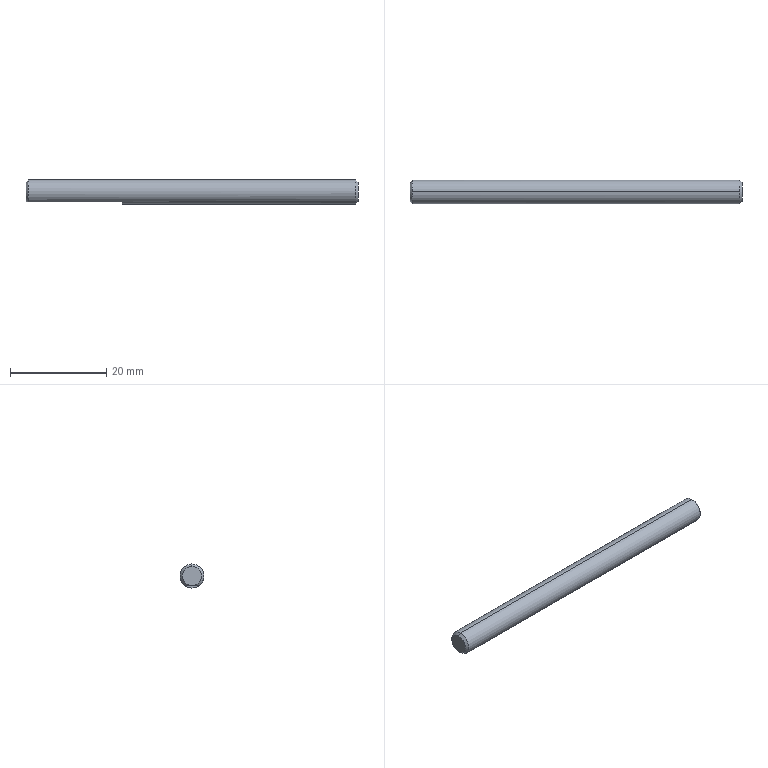Part | SolidWorks | features BaseBody 1 | 1 solid | 10 faces | box 69 x 5 x 5 mm | volume 1331 mm3 | cone 4 | plane 4 | cylinder 2 | commonest cylinder face diameters 5 x2
STEP:
#1=CARTESIAN_POINT('',(69.,0.,-2.));
#2=VERTEX_POINT('',#1);
#3=CARTESIAN_POINT('',(69.,0.,2.));
#4=VERTEX_POINT('',#3);
#5=CARTESIAN_POINT('',(69.,0.,0.));
#6=DIRECTION('',(1.,0.,0.));
#7=DIRECTION('',(0.,0.,1.));
#8=AXIS2_PLACEMENT_3D('',#5,#6,#7);
#9=CIRCLE('',#8,2.);
#10=EDGE_CURVE('',#2,#4,#9,.T.);
#11=ORIENTED_EDGE('',*,*,#10,.F.);
#12=CARTESIAN_POINT('',(68.5,0.,-2.5));
#13=VERTEX_POINT('',#12);
#14=CARTESIAN_POINT('',(69.,0.,-2.));
#15=DIRECTION('',(-0.7071,0.,-0.7071));
#16=VECTOR('',#15,1000.);
#17=LINE('',#14,#16);
#18=EDGE_CURVE('',#2,#13,#17,.T.);
#19=ORIENTED_EDGE('',*,*,#18,.T.);
#20=CARTESIAN_POINT('',(68.5,0.,2.5));
#21=VERTEX_POINT('',#20);
#22=CARTESIAN_POINT('',(68.5,0.,0.));
#23=DIRECTION('',(-1.,0.,0.));
#24=DIRECTION('',(0.,0.,1.));
#25=AXIS2_PLACEMENT_3D('',#22,#23,#24);
#26=CIRCLE('',#25,2.5);
#27=EDGE_CURVE('',#21,#13,#26,.T.);
#28=ORIENTED_EDGE('',*,*,#27,.F.);
#29=CARTESIAN_POINT('',(69.,0.,2.));
#30=DIRECTION('',(-0.7071,0.,0.7071));
#31=VECTOR('',#30,1000.);
#32=LINE('',#29,#31);
#33=EDGE_CURVE('',#4,#21,#32,.T.);
#34=ORIENTED_EDGE('',*,*,#33,.F.);
#35=EDGE_LOOP('',(#11,#19,#28,#34));
#36=FACE_OUTER_BOUND('',#35,.T.);
#37=CARTESIAN_POINT('',(69.,0.,0.));
#38=DIRECTION('',(-1.,0.,0.));
#39=DIRECTION('',(0.,0.,1.));
#40=AXIS2_PLACEMENT_3D('',#37,#38,#39);
#41=CONICAL_SURFACE('',#40,2.,0.7854);
#42=ADVANCED_FACE('',(#36),#41,.T.);
#43=ORIENTED_EDGE('',*,*,#27,.T.);
#44=CARTESIAN_POINT('',(20.,0.,-2.5));
#45=VERTEX_POINT('',#44);
#46=CARTESIAN_POINT('',(68.5,0.,-2.5));
#47=DIRECTION('',(-1.,0.,0.));
#48=VECTOR('',#47,1000.);
#49=LINE('',#46,#48);
#50=EDGE_CURVE('',#13,#45,#49,.T.);
#51=ORIENTED_EDGE('',*,*,#50,.T.);
#52=CARTESIAN_POINT('',(20.,1.5,-2.));
#53=VERTEX_POINT('',#52);
#54=CARTESIAN_POINT('',(20.,0.,0.));
#55=DIRECTION('',(-1.,0.,0.));
#56=DIRECTION('',(0.,0.,1.));
#57=AXIS2_PLACEMENT_3D('',#54,#55,#56);
#58=CIRCLE('',#57,2.5);
#59=EDGE_CURVE('',#53,#45,#58,.T.);
#60=ORIENTED_EDGE('',*,*,#59,.F.);
#61=CARTESIAN_POINT('',(0.5,1.5,-2.));
#62=VERTEX_POINT('',#61);
#63=CARTESIAN_POINT('',(34.5,1.5,-2.));
#64=DIRECTION('',(1.,0.,0.));
#65=VECTOR('',#64,1000.);
#66=LINE('',#63,#65);
#67=EDGE_CURVE('',#62,#53,#66,.T.);
#68=ORIENTED_EDGE('',*,*,#67,.F.);
#69=CARTESIAN_POINT('',(0.5,0.,2.5));
#70=VERTEX_POINT('',#69);
#71=CARTESIAN_POINT('',(0.5,0.,0.));
#72=DIRECTION('',(-1.,0.,0.));
#73=DIRECTION('',(0.,0.,1.));
#74=AXIS2_PLACEMENT_3D('',#71,#72,#73);
#75=CIRCLE('',#74,2.5);
#76=EDGE_CURVE('',#70,#62,#75,.T.);
#77=ORIENTED_EDGE('',*,*,#76,.F.);
#78=CARTESIAN_POINT('',(68.5,0.,2.5));
#79=DIRECTION('',(-1.,0.,0.));
#80=VECTOR('',#79,1000.);
#81=LINE('',#78,#80);
#82=EDGE_CURVE('',#21,#70,#81,.T.);
#83=ORIENTED_EDGE('',*,*,#82,.F.);
#84=EDGE_LOOP('',(#43,#51,#60,#68,#77,#83));
#85=FACE_OUTER_BOUND('',#84,.T.);
#86=CARTESIAN_POINT('',(68.5,0.,0.));
#87=DIRECTION('',(-1.,0.,0.));
#88=DIRECTION('',(0.,0.,1.));
#89=AXIS2_PLACEMENT_3D('',#86,#87,#88);
#90=CYLINDRICAL_SURFACE('',#89,2.5);
#91=ADVANCED_FACE('',(#85),#90,.T.);
#92=CARTESIAN_POINT('',(0.,0.,2.));
#93=VERTEX_POINT('',#92);
#94=CARTESIAN_POINT('',(0.,0.,-2.));
#95=VERTEX_POINT('',#94);
#96=CARTESIAN_POINT('',(0.,0.,0.));
#97=DIRECTION('',(-1.,0.,0.));
#98=DIRECTION('',(0.,0.,-1.));
#99=AXIS2_PLACEMENT_3D('',#96,#97,#98);
#100=CIRCLE('',#99,2.);
#101=EDGE_CURVE('',#93,#95,#100,.T.);
#102=ORIENTED_EDGE('',*,*,#101,.F.);
#103=CARTESIAN_POINT('',(0.,0.,2.));
#104=DIRECTION('',(0.7071,0.,0.7071));
#105=VECTOR('',#104,1000.);
#106=LINE('',#103,#105);
#107=EDGE_CURVE('',#93,#70,#106,.T.);
#108=ORIENTED_EDGE('',*,*,#107,.T.);
#109=ORIENTED_EDGE('',*,*,#76,.T.);
#110=CARTESIAN_POINT('',(0.5,1.5,-2.));
#111=CARTESIAN_POINT('',(0.4247,1.374,-2.));
#112=CARTESIAN_POINT('',(0.3577,1.253,-2.));
#113=CARTESIAN_POINT('',(0.2697,1.074,-2.));
#114=CARTESIAN_POINT('',(0.2425,1.016,-2.));
#115=CARTESIAN_POINT('',(0.2048,0.9284,-2.));
#116=CARTESIAN_POINT('',(0.1867,0.8849,-2.));
#117=CARTESIAN_POINT('',(0.1698,0.8417,-2.));
#118=CARTESIAN_POINT('',(0.1588,0.8129,-2.));
#119=CARTESIAN_POINT('',(0.1542,0.8005,-2.));
#120=CARTESIAN_POINT('',(0.1244,0.7188,-2.));
#121=CARTESIAN_POINT('',(0.1034,0.6543,-2.));
#122=CARTESIAN_POINT('',(0.07615,0.558,-2.));
#123=CARTESIAN_POINT('',(0.06778,0.526,-2.));
#124=CARTESIAN_POINT('',(0.05245,0.4621,-2.));
#125=CARTESIAN_POINT('',(0.0458,0.4317,-2.));
#126=CARTESIAN_POINT('',(0.01309,0.2642,-2.));
#127=CARTESIAN_POINT('',(0.,0.1332,-2.));
#128=CARTESIAN_POINT('',(0.,0.,-2.));
#129=B_SPLINE_CURVE_WITH_KNOTS('',3,(#110,#111,#112,#113,#114,#115,#116,#117,#118,#119,#120,#121,#122,#123,#124,#125,#126,#127,#128),.UNSPECIFIED.,.F.,.F.,(4,2,2,1,2,2,2,2,2,4),(0.,0.25,0.375,0.4375,0.4688,0.5,0.625,0.6875,0.75,1.),.UNSPECIFIED.);
#130=EDGE_CURVE('',#62,#95,#129,.T.);
#131=ORIENTED_EDGE('',*,*,#130,.T.);
#132=EDGE_LOOP('',(#102,#108,#109,#131));
#133=FACE_OUTER_BOUND('',#132,.T.);
#134=CARTESIAN_POINT('',(0.,0.,0.));
#135=DIRECTION('',(1.,0.,0.));
#136=DIRECTION('',(0.,0.,-1.));
#137=AXIS2_PLACEMENT_3D('',#134,#135,#136);
#138=CONICAL_SURFACE('',#137,2.,0.7854);
#139=ADVANCED_FACE('',(#133),#138,.T.);
#140=CARTESIAN_POINT('',(0.,0.,0.));
#141=DIRECTION('',(-1.,0.,0.));
#142=DIRECTION('',(0.,0.,-1.));
#143=AXIS2_PLACEMENT_3D('',#140,#141,#142);
#144=CIRCLE('',#143,2.);
#145=EDGE_CURVE('',#95,#93,#144,.T.);
#146=ORIENTED_EDGE('',*,*,#145,.T.);
#147=ORIENTED_EDGE('',*,*,#101,.T.);
#148=EDGE_LOOP('',(#146,#147));
#149=FACE_OUTER_BOUND('',#148,.T.);
#150=CARTESIAN_POINT('',(0.,-2.024,2.024));
#151=DIRECTION('',(1.,0.,0.));
#152=DIRECTION('',(0.,1.,0.));
#153=AXIS2_PLACEMENT_3D('',#150,#151,#152);
#154=PLANE('',#153);
#155=ADVANCED_FACE('',(#149),#154,.F.);
#156=ORIENTED_EDGE('',*,*,#59,.T.);
#157=CARTESIAN_POINT('',(20.,-1.5,-2.));
#158=VERTEX_POINT('',#157);
#159=CARTESIAN_POINT('',(20.,0.,0.));
#160=DIRECTION('',(-1.,0.,0.));
#161=DIRECTION('',(0.,0.,1.));
#162=AXIS2_PLACEMENT_3D('',#159,#160,#161);
#163=CIRCLE('',#162,2.5);
#164=EDGE_CURVE('',#45,#158,#163,.T.);
#165=ORIENTED_EDGE('',*,*,#164,.T.);
#166=CARTESIAN_POINT('',(20.,0.,-2.));
#167=DIRECTION('',(0.,1.,0.));
#168=VECTOR('',#167,1000.);
#169=LINE('',#166,#168);
#170=EDGE_CURVE('',#158,#53,#169,.T.);
#171=ORIENTED_EDGE('',*,*,#170,.T.);
#172=EDGE_LOOP('',(#156,#165,#171));
#173=FACE_OUTER_BOUND('',#172,.T.);
#174=CARTESIAN_POINT('',(20.,-1.518,-2.503));
#175=DIRECTION('',(-1.,0.,0.));
#176=DIRECTION('',(0.,0.,1.));
#177=AXIS2_PLACEMENT_3D('',#174,#175,#176);
#178=PLANE('',#177);
#179=ADVANCED_FACE('',(#173),#178,.T.);
#180=ORIENTED_EDGE('',*,*,#107,.F.);
#181=ORIENTED_EDGE('',*,*,#145,.F.);
#182=CARTESIAN_POINT('',(0.5,-1.5,-2.));
#183=VERTEX_POINT('',#182);
#184=CARTESIAN_POINT('',(0.,0.,-2.));
#185=CARTESIAN_POINT('',(0.,-0.06627,-2.));
#186=CARTESIAN_POINT('',(0.003273,-0.1321,-2.));
#187=CARTESIAN_POINT('',(0.01309,-0.2312,-2.));
#188=CARTESIAN_POINT('',(0.01718,-0.2643,-2.));
#189=CARTESIAN_POINT('',(0.027,-0.3308,-2.));
#190=CARTESIAN_POINT('',(0.03306,-0.3659,-2.));
#191=CARTESIAN_POINT('',(0.05171,-0.4615,-2.));
#192=CARTESIAN_POINT('',(0.06695,-0.5252,-2.));
#193=CARTESIAN_POINT('',(0.09401,-0.6211,-2.));
#194=CARTESIAN_POINT('',(0.1086,-0.6691,-2.));
#195=CARTESIAN_POINT('',(0.1247,-0.7175,-2.));
#196=CARTESIAN_POINT('',(0.1359,-0.7498,-2.));
#197=CARTESIAN_POINT('',(0.1423,-0.7678,-2.));
#198=CARTESIAN_POINT('',(0.2314,-1.012,-2.));
#199=CARTESIAN_POINT('',(0.3489,-1.248,-2.));
#200=CARTESIAN_POINT('',(0.5,-1.5,-2.));
#201=B_SPLINE_CURVE_WITH_KNOTS('',3,(#184,#185,#186,#187,#188,#189,#190,#191,#192,#193,#194,#195,#196,#197,#198,#199,#200),.UNSPECIFIED.,.F.,.F.,(4,2,2,2,2,1,2,2,4),(0.,0.125,0.1875,0.25,0.375,0.4375,0.4688,0.5,1.),.UNSPECIFIED.);
#202=EDGE_CURVE('',#95,#183,#201,.T.);
#203=ORIENTED_EDGE('',*,*,#202,.T.);
#204=CARTESIAN_POINT('',(0.5,0.,0.));
#205=DIRECTION('',(-1.,0.,0.));
#206=DIRECTION('',(0.,0.,1.));
#207=AXIS2_PLACEMENT_3D('',#204,#205,#206);
#208=CIRCLE('',#207,2.5);
#209=EDGE_CURVE('',#183,#70,#208,.T.);
#210=ORIENTED_EDGE('',*,*,#209,.T.);
#211=EDGE_LOOP('',(#180,#181,#203,#210));
#212=FACE_OUTER_BOUND('',#211,.T.);
#213=CARTESIAN_POINT('',(0.,0.,0.));
#214=DIRECTION('',(1.,0.,0.));
#215=DIRECTION('',(0.,0.,-1.));
#216=AXIS2_PLACEMENT_3D('',#213,#214,#215);
#217=CONICAL_SURFACE('',#216,2.,0.7854);
#218=ADVANCED_FACE('',(#212),#217,.T.);
#219=ORIENTED_EDGE('',*,*,#170,.F.);
#220=CARTESIAN_POINT('',(34.5,-1.5,-2.));
#221=DIRECTION('',(-1.,0.,0.));
#222=VECTOR('',#221,1000.);
#223=LINE('',#220,#222);
#224=EDGE_CURVE('',#158,#183,#223,.T.);
#225=ORIENTED_EDGE('',*,*,#224,.T.);
#226=ORIENTED_EDGE('',*,*,#202,.F.);
#227=ORIENTED_EDGE('',*,*,#130,.F.);
#228=ORIENTED_EDGE('',*,*,#67,.T.);
#229=EDGE_LOOP('',(#219,#225,#226,#227,#228));
#230=FACE_OUTER_BOUND('',#229,.T.);
#231=CARTESIAN_POINT('',(-0.12,-1.5,-2.));
#232=DIRECTION('',(0.,0.,1.));
#233=DIRECTION('',(1.,0.,0.));
#234=AXIS2_PLACEMENT_3D('',#231,#232,#233);
#235=PLANE('',#234);
#236=ADVANCED_FACE('',(#230),#235,.F.);
#237=ORIENTED_EDGE('',*,*,#50,.F.);
#238=CARTESIAN_POINT('',(68.5,0.,0.));
#239=DIRECTION('',(-1.,0.,0.));
#240=DIRECTION('',(0.,0.,1.));
#241=AXIS2_PLACEMENT_3D('',#238,#239,#240);
#242=CIRCLE('',#241,2.5);
#243=EDGE_CURVE('',#13,#21,#242,.T.);
#244=ORIENTED_EDGE('',*,*,#243,.T.);
#245=ORIENTED_EDGE('',*,*,#82,.T.);
#246=ORIENTED_EDGE('',*,*,#209,.F.);
#247=ORIENTED_EDGE('',*,*,#224,.F.);
#248=ORIENTED_EDGE('',*,*,#164,.F.);
#249=EDGE_LOOP('',(#237,#244,#245,#246,#247,#248));
#250=FACE_OUTER_BOUND('',#249,.T.);
#251=CARTESIAN_POINT('',(68.5,0.,0.));
#252=DIRECTION('',(-1.,0.,0.));
#253=DIRECTION('',(0.,0.,1.));
#254=AXIS2_PLACEMENT_3D('',#251,#252,#253);
#255=CYLINDRICAL_SURFACE('',#254,2.5);
#256=ADVANCED_FACE('',(#250),#255,.T.);
#257=CARTESIAN_POINT('',(69.,0.,0.));
#258=DIRECTION('',(1.,0.,0.));
#259=DIRECTION('',(0.,0.,1.));
#260=AXIS2_PLACEMENT_3D('',#257,#258,#259);
#261=CIRCLE('',#260,2.);
#262=EDGE_CURVE('',#4,#2,#261,.T.);
#263=ORIENTED_EDGE('',*,*,#262,.T.);
#264=ORIENTED_EDGE('',*,*,#10,.T.);
#265=EDGE_LOOP('',(#263,#264));
#266=FACE_OUTER_BOUND('',#265,.T.);
#267=CARTESIAN_POINT('',(69.,-2.024,-2.024));
#268=DIRECTION('',(-1.,0.,0.));
#269=DIRECTION('',(0.,0.,1.));
#270=AXIS2_PLACEMENT_3D('',#267,#268,#269);
#271=PLANE('',#270);
#272=ADVANCED_FACE('',(#266),#271,.F.);
#273=ORIENTED_EDGE('',*,*,#18,.F.);
#274=ORIENTED_EDGE('',*,*,#262,.F.);
#275=ORIENTED_EDGE('',*,*,#33,.T.);
#276=ORIENTED_EDGE('',*,*,#243,.F.);
#277=EDGE_LOOP('',(#273,#274,#275,#276));
#278=FACE_OUTER_BOUND('',#277,.T.);
#279=CARTESIAN_POINT('',(69.,0.,0.));
#280=DIRECTION('',(-1.,0.,0.));
#281=DIRECTION('',(0.,0.,1.));
#282=AXIS2_PLACEMENT_3D('',#279,#280,#281);
#283=CONICAL_SURFACE('',#282,2.,0.7854);
#284=ADVANCED_FACE('',(#278),#283,.T.);
#285=CLOSED_SHELL('',(#42,#91,#139,#155,#179,#218,#236,#256,#272,#284));
#286=MANIFOLD_SOLID_BREP('',#285);
#287=CARTESIAN_POINT('',(0.,0.,0.));
#288=DIRECTION('',(0.,0.,1.));
#289=DIRECTION('',(1.,0.,0.));
#290=AXIS2_PLACEMENT_3D('',#287,#288,#289);
#291=(LENGTH_UNIT()NAMED_UNIT(*)SI_UNIT(.MILLI.,.METRE.));
#292=UNCERTAINTY_MEASURE_WITH_UNIT(LENGTH_MEASURE(0.00001),#291,'','');
#293=(NAMED_UNIT(*)PLANE_ANGLE_UNIT()SI_UNIT($,.RADIAN.));
#294=(NAMED_UNIT(*)SI_UNIT($,.STERADIAN.)SOLID_ANGLE_UNIT());
#295=(GEOMETRIC_REPRESENTATION_CONTEXT(3)GLOBAL_UNCERTAINTY_ASSIGNED_CONTEXT((#292))GLOBAL_UNIT_ASSIGNED_CONTEXT((#291,#293,#294))REPRESENTATION_CONTEXT('',''));
#296=ADVANCED_BREP_SHAPE_REPRESENTATION('',(#286,#290),#295);